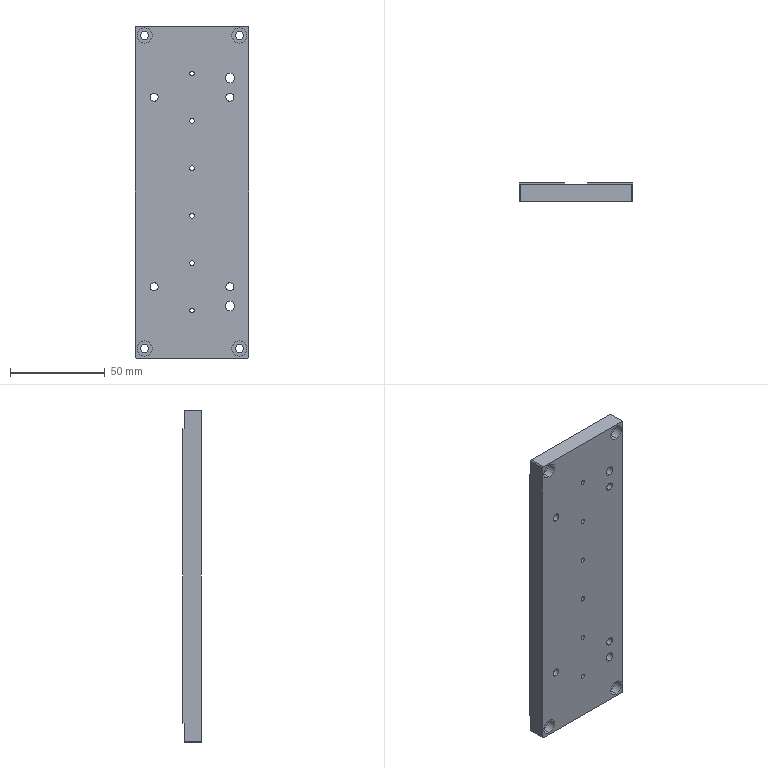Part | STEP file | PN_0047 Mount electronic clip mounting base plate | 1 solid | 68 faces | box 60 x 10 x 175 mm | volume 99342 mm3 | cylinder 44 | plane 24 | commonest cylinder face diameters 2.5 x12 4.2 x8 4.3 x8 8 x8 4 x4 5 x4